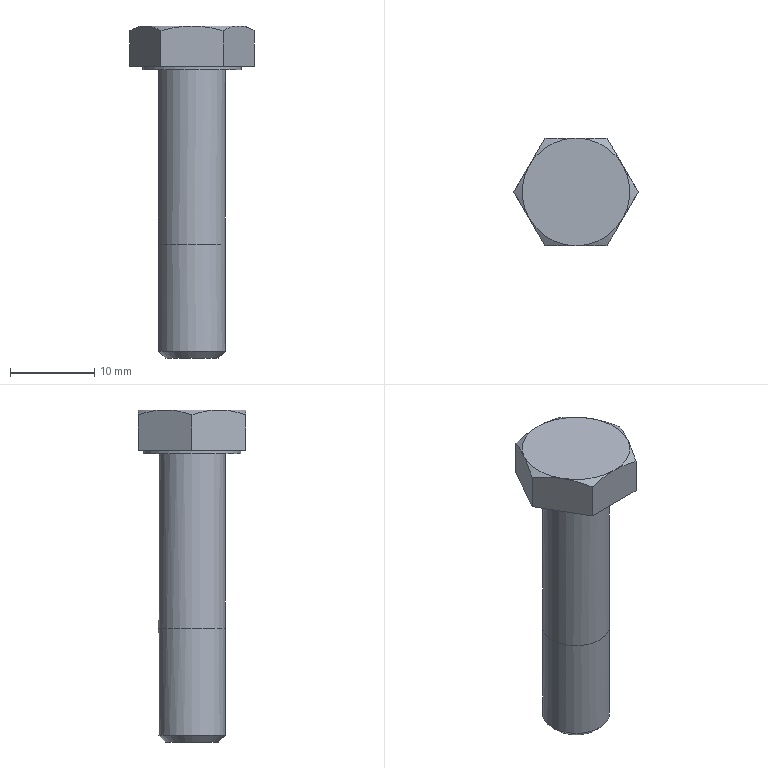Part | NX | features solid 2 | 1 solid | 20 faces | box 14.723 x 12.751 x 39.313 mm | volume 2395 mm3 | plane 10 | cone 7 | cylinder 3 | commonest cylinder face diameters 7.938 x2 11.684 x1
STEP:
#1=CARTESIAN_POINT('',(-3.969,0.,-5.182));
#2=VERTEX_POINT('',#1);
#3=CARTESIAN_POINT('',(0.,0.,-5.182));
#4=DIRECTION('',(0.,0.,-1.));
#5=DIRECTION('',(-1.,0.,0.));
#6=AXIS2_PLACEMENT_3D('',#3,#4,#5);
#7=CIRCLE('',#6,3.969);
#8=EDGE_CURVE('',#2,#2,#7,.T.);
#9=ORIENTED_EDGE('',*,*,#8,.T.);
#10=EDGE_LOOP('',(#9));
#11=FACE_BOUND('',#10,.T.);
#12=CARTESIAN_POINT('',(-3.969,0.,-25.819));
#13=VERTEX_POINT('',#12);
#14=CARTESIAN_POINT('',(-3.11,3.11,-25.819));
#15=CARTESIAN_POINT('',(-4.398,0.,-25.819));
#16=CARTESIAN_POINT('',(-3.11,-3.11,-25.819));
#17=CARTESIAN_POINT('',(0.,-4.398,-25.819));
#18=CARTESIAN_POINT('',(3.11,-3.11,-25.819));
#19=CARTESIAN_POINT('',(4.398,0.,-25.819));
#20=CARTESIAN_POINT('',(3.11,3.11,-25.819));
#21=CARTESIAN_POINT('',(0.,4.398,-25.819));
#22=CARTESIAN_POINT('',(-3.11,3.11,-25.819));
#23=CARTESIAN_POINT('',(-4.398,0.,-25.819));
#24=CARTESIAN_POINT('',(-3.11,-3.11,-25.819));
#25=B_SPLINE_CURVE_WITH_KNOTS('',3,(#14,#15,#16,#17,#18,#19,#20,#21,#22,#23,#24),.UNSPECIFIED.,.T.,.F.,(1,1,1,1,1,1,1,1,1,1,1,1,1,1,1),(-0.375,-0.25,-0.125,0.,0.125,0.25,0.375,0.5,0.625,0.75,0.875,1.,1.125,1.25,1.375),.UNSPECIFIED.);
#26=EDGE_CURVE('',#13,#13,#25,.T.);
#27=ORIENTED_EDGE('',*,*,#26,.T.);
#28=EDGE_LOOP('',(#27));
#29=FACE_BOUND('',#28,.T.);
#30=CARTESIAN_POINT('',(0.,0.,0.));
#31=DIRECTION('',(0.,0.,-1.));
#32=DIRECTION('',(-1.,0.,0.));
#33=AXIS2_PLACEMENT_3D('',#30,#31,#32);
#34=CYLINDRICAL_SURFACE('',#33,3.969);
#35=ADVANCED_FACE('',(#11,#29),#34,.T.);
#36=CARTESIAN_POINT('',(-7.362,0.,-4.775));
#37=VERTEX_POINT('',#36);
#38=CARTESIAN_POINT('',(-3.681,6.375,-4.775));
#39=VERTEX_POINT('',#38);
#40=CARTESIAN_POINT('',(-4.061,5.717,-4.775));
#41=DIRECTION('',(0.5,0.866,0.));
#42=VECTOR('',#41,1000.);
#43=LINE('',#40,#42);
#44=EDGE_CURVE('',#37,#39,#43,.T.);
#45=ORIENTED_EDGE('',*,*,#44,.T.);
#46=CARTESIAN_POINT('',(3.681,6.375,-4.775));
#47=VERTEX_POINT('',#46);
#48=CARTESIAN_POINT('',(5.842,6.375,-4.775));
#49=DIRECTION('',(1.,0.,0.));
#50=VECTOR('',#49,1000.);
#51=LINE('',#48,#50);
#52=EDGE_CURVE('',#39,#47,#51,.T.);
#53=ORIENTED_EDGE('',*,*,#52,.T.);
#54=CARTESIAN_POINT('',(7.362,0.,-4.775));
#55=VERTEX_POINT('',#54);
#56=CARTESIAN_POINT('',(6.982,0.658,-4.775));
#57=DIRECTION('',(0.5,-0.866,0.));
#58=VECTOR('',#57,1000.);
#59=LINE('',#56,#58);
#60=EDGE_CURVE('',#47,#55,#59,.T.);
#61=ORIENTED_EDGE('',*,*,#60,.T.);
#62=CARTESIAN_POINT('',(3.681,-6.375,-4.775));
#63=VERTEX_POINT('',#62);
#64=CARTESIAN_POINT('',(6.982,-0.658,-4.775));
#65=DIRECTION('',(-0.5,-0.866,0.));
#66=VECTOR('',#65,1000.);
#67=LINE('',#64,#66);
#68=EDGE_CURVE('',#55,#63,#67,.T.);
#69=ORIENTED_EDGE('',*,*,#68,.T.);
#70=CARTESIAN_POINT('',(-3.681,-6.375,-4.775));
#71=VERTEX_POINT('',#70);
#72=CARTESIAN_POINT('',(5.842,-6.375,-4.775));
#73=DIRECTION('',(-1.,0.,0.));
#74=VECTOR('',#73,1000.);
#75=LINE('',#72,#74);
#76=EDGE_CURVE('',#63,#71,#75,.T.);
#77=ORIENTED_EDGE('',*,*,#76,.T.);
#78=CARTESIAN_POINT('',(-4.061,-5.717,-4.775));
#79=DIRECTION('',(-0.5,0.866,0.));
#80=VECTOR('',#79,1000.);
#81=LINE('',#78,#80);
#82=EDGE_CURVE('',#71,#37,#81,.T.);
#83=ORIENTED_EDGE('',*,*,#82,.T.);
#84=EDGE_LOOP('',(#45,#53,#61,#69,#77,#83));
#85=FACE_BOUND('',#84,.T.);
#86=CARTESIAN_POINT('',(-5.842,0.,-4.775));
#87=VERTEX_POINT('',#86);
#88=CARTESIAN_POINT('',(0.,0.,-4.775));
#89=DIRECTION('',(0.,0.,-1.));
#90=DIRECTION('',(-1.,0.,0.));
#91=AXIS2_PLACEMENT_3D('',#88,#89,#90);
#92=CIRCLE('',#91,5.842);
#93=EDGE_CURVE('',#87,#87,#92,.T.);
#94=ORIENTED_EDGE('',*,*,#93,.F.);
#95=EDGE_LOOP('',(#94));
#96=FACE_BOUND('',#95,.T.);
#97=CARTESIAN_POINT('',(5.842,0.,-4.775));
#98=DIRECTION('',(0.,0.,-1.));
#99=DIRECTION('',(-1.,0.,0.));
#100=AXIS2_PLACEMENT_3D('',#97,#98,#99);
#101=PLANE('',#100);
#102=ADVANCED_FACE('',(#85,#96),#101,.T.);
#103=CARTESIAN_POINT('',(-3.181,0.,-39.313));
#104=VERTEX_POINT('',#103);
#105=CARTESIAN_POINT('',(0.,0.,-39.313));
#106=DIRECTION('',(0.,0.,-1.));
#107=DIRECTION('',(-1.,0.,0.));
#108=AXIS2_PLACEMENT_3D('',#105,#106,#107);
#109=CIRCLE('',#108,3.181);
#110=EDGE_CURVE('',#104,#104,#109,.T.);
#111=ORIENTED_EDGE('',*,*,#110,.T.);
#112=EDGE_LOOP('',(#111));
#113=FACE_BOUND('',#112,.T.);
#114=CARTESIAN_POINT('',(0.,0.,-39.313));
#115=DIRECTION('',(0.,0.,-1.));
#116=DIRECTION('',(-1.,0.,0.));
#117=AXIS2_PLACEMENT_3D('',#114,#115,#116);
#118=PLANE('',#117);
#119=ADVANCED_FACE('',(#113),#118,.T.);
#120=CARTESIAN_POINT('',(-3.969,0.,-38.525));
#121=VERTEX_POINT('',#120);
#122=CARTESIAN_POINT('',(0.,0.,-38.525));
#123=DIRECTION('',(0.,0.,-1.));
#124=DIRECTION('',(-1.,0.,0.));
#125=AXIS2_PLACEMENT_3D('',#122,#123,#124);
#126=CIRCLE('',#125,3.969);
#127=EDGE_CURVE('',#121,#121,#126,.T.);
#128=ORIENTED_EDGE('',*,*,#127,.T.);
#129=EDGE_LOOP('',(#128));
#130=FACE_BOUND('',#129,.T.);
#131=ORIENTED_EDGE('',*,*,#110,.F.);
#132=EDGE_LOOP('',(#131));
#133=FACE_BOUND('',#132,.T.);
#134=CARTESIAN_POINT('',(0.,0.,-39.313));
#135=DIRECTION('',(0.,0.,1.));
#136=DIRECTION('',(1.,0.,0.));
#137=AXIS2_PLACEMENT_3D('',#134,#135,#136);
#138=CONICAL_SURFACE('',#137,3.181,0.7854);
#139=ADVANCED_FACE('',(#130,#133),#138,.T.);
#140=ORIENTED_EDGE('',*,*,#26,.F.);
#141=EDGE_LOOP('',(#140));
#142=FACE_BOUND('',#141,.T.);
#143=ORIENTED_EDGE('',*,*,#127,.F.);
#144=EDGE_LOOP('',(#143));
#145=FACE_BOUND('',#144,.T.);
#146=CARTESIAN_POINT('',(0.,0.,0.));
#147=DIRECTION('',(0.,0.,-1.));
#148=DIRECTION('',(-1.,0.,0.));
#149=AXIS2_PLACEMENT_3D('',#146,#147,#148);
#150=CYLINDRICAL_SURFACE('',#149,3.969);
#151=ADVANCED_FACE('',(#142,#145),#150,.T.);
#152=CARTESIAN_POINT('',(-5.842,0.,-5.182));
#153=VERTEX_POINT('',#152);
#154=CARTESIAN_POINT('',(0.,0.,-5.182));
#155=DIRECTION('',(0.,0.,-1.));
#156=DIRECTION('',(-1.,0.,0.));
#157=AXIS2_PLACEMENT_3D('',#154,#155,#156);
#158=CIRCLE('',#157,5.842);
#159=EDGE_CURVE('',#153,#153,#158,.T.);
#160=ORIENTED_EDGE('',*,*,#159,.T.);
#161=EDGE_LOOP('',(#160));
#162=FACE_BOUND('',#161,.T.);
#163=ORIENTED_EDGE('',*,*,#8,.F.);
#164=EDGE_LOOP('',(#163));
#165=FACE_BOUND('',#164,.T.);
#166=CARTESIAN_POINT('',(3.969,0.,-5.182));
#167=DIRECTION('',(0.,0.,-1.));
#168=DIRECTION('',(-1.,0.,0.));
#169=AXIS2_PLACEMENT_3D('',#166,#167,#168);
#170=PLANE('',#169);
#171=ADVANCED_FACE('',(#162,#165),#170,.T.);
#172=ORIENTED_EDGE('',*,*,#93,.T.);
#173=EDGE_LOOP('',(#172));
#174=FACE_BOUND('',#173,.T.);
#175=ORIENTED_EDGE('',*,*,#159,.F.);
#176=EDGE_LOOP('',(#175));
#177=FACE_BOUND('',#176,.T.);
#178=CARTESIAN_POINT('',(0.,0.,0.));
#179=DIRECTION('',(0.,0.,-1.));
#180=DIRECTION('',(-1.,0.,0.));
#181=AXIS2_PLACEMENT_3D('',#178,#179,#180);
#182=CYLINDRICAL_SURFACE('',#181,5.842);
#183=ADVANCED_FACE('',(#174,#177),#182,.T.);
#184=ORIENTED_EDGE('',*,*,#52,.F.);
#185=CARTESIAN_POINT('',(-3.681,6.375,-0.5694));
#186=VERTEX_POINT('',#185);
#187=CARTESIAN_POINT('',(-3.681,6.375,-43.244));
#188=DIRECTION('',(0.,0.,1.));
#189=VECTOR('',#188,1000.);
#190=LINE('',#187,#189);
#191=EDGE_CURVE('',#39,#186,#190,.T.);
#192=ORIENTED_EDGE('',*,*,#191,.T.);
#193=CARTESIAN_POINT('',(0.,6.375,0.));
#194=VERTEX_POINT('',#193);
#195=CARTESIAN_POINT('',(-3.681,6.375,-0.5694));
#196=CARTESIAN_POINT('',(-2.484,6.375,-0.2238));
#197=CARTESIAN_POINT('',(-1.244,6.375,0.));
#198=CARTESIAN_POINT('',(0.,6.375,0.));
#199=B_SPLINE_CURVE_WITH_KNOTS('',3,(#195,#196,#197,#198),.UNSPECIFIED.,.F.,.F.,(4,4),(0.006567,0.01029),.UNSPECIFIED.);
#200=EDGE_CURVE('',#194,#186,#199,.F.);
#201=ORIENTED_EDGE('',*,*,#200,.F.);
#202=CARTESIAN_POINT('',(3.681,6.375,-0.5694));
#203=VERTEX_POINT('',#202);
#204=CARTESIAN_POINT('',(0.,6.375,0.));
#205=CARTESIAN_POINT('',(1.245,6.375,0.));
#206=CARTESIAN_POINT('',(2.49,6.375,-0.2258));
#207=CARTESIAN_POINT('',(3.681,6.375,-0.5694));
#208=B_SPLINE_CURVE_WITH_KNOTS('',3,(#204,#205,#206,#207),.UNSPECIFIED.,.F.,.F.,(4,4),(0.01029,0.01402),.UNSPECIFIED.);
#209=EDGE_CURVE('',#203,#194,#208,.F.);
#210=ORIENTED_EDGE('',*,*,#209,.F.);
#211=CARTESIAN_POINT('',(3.681,6.375,-43.244));
#212=DIRECTION('',(0.,0.,1.));
#213=VECTOR('',#212,1000.);
#214=LINE('',#211,#213);
#215=EDGE_CURVE('',#47,#203,#214,.T.);
#216=ORIENTED_EDGE('',*,*,#215,.F.);
#217=EDGE_LOOP('',(#184,#192,#201,#210,#216));
#218=FACE_BOUND('',#217,.T.);
#219=CARTESIAN_POINT('',(3.681,6.375,-43.244));
#220=DIRECTION('',(0.,1.,0.));
#221=DIRECTION('',(0.,0.,1.));
#222=AXIS2_PLACEMENT_3D('',#219,#220,#221);
#223=PLANE('',#222);
#224=ADVANCED_FACE('',(#218),#223,.T.);
#225=ORIENTED_EDGE('',*,*,#44,.F.);
#226=CARTESIAN_POINT('',(-7.362,0.,-0.5694));
#227=VERTEX_POINT('',#226);
#228=CARTESIAN_POINT('',(-7.362,0.,-43.244));
#229=DIRECTION('',(0.,0.,1.));
#230=VECTOR('',#229,1000.);
#231=LINE('',#228,#230);
#232=EDGE_CURVE('',#37,#227,#231,.T.);
#233=ORIENTED_EDGE('',*,*,#232,.T.);
#234=CARTESIAN_POINT('',(-5.521,3.188,0.));
#235=VERTEX_POINT('',#234);
#236=CARTESIAN_POINT('',(-5.521,3.188,0.));
#237=CARTESIAN_POINT('',(-6.146,2.106,0.));
#238=CARTESIAN_POINT('',(-6.761,1.04,-0.2227));
#239=CARTESIAN_POINT('',(-7.362,0.,-0.5694));
#240=B_SPLINE_CURVE_WITH_KNOTS('',3,(#236,#237,#238,#239),.UNSPECIFIED.,.F.,.F.,(4,4),(0.003725,0.007435),.UNSPECIFIED.);
#241=EDGE_CURVE('',#235,#227,#240,.T.);
#242=ORIENTED_EDGE('',*,*,#241,.F.);
#243=CARTESIAN_POINT('',(-3.681,6.375,-0.5694));
#244=CARTESIAN_POINT('',(-4.283,5.332,-0.2218));
#245=CARTESIAN_POINT('',(-4.894,4.274,0.));
#246=CARTESIAN_POINT('',(-5.521,3.188,0.));
#247=B_SPLINE_CURVE_WITH_KNOTS('',3,(#243,#244,#245,#246),.UNSPECIFIED.,.F.,.F.,(4,4),(0.000000238,0.003725),.UNSPECIFIED.);
#248=EDGE_CURVE('',#186,#235,#247,.T.);
#249=ORIENTED_EDGE('',*,*,#248,.F.);
#250=ORIENTED_EDGE('',*,*,#191,.F.);
#251=EDGE_LOOP('',(#225,#233,#242,#249,#250));
#252=FACE_BOUND('',#251,.T.);
#253=CARTESIAN_POINT('',(-3.681,6.375,-43.244));
#254=DIRECTION('',(-0.866,0.5,0.));
#255=DIRECTION('',(-0.5,-0.866,0.));
#256=AXIS2_PLACEMENT_3D('',#253,#254,#255);
#257=PLANE('',#256);
#258=ADVANCED_FACE('',(#252),#257,.T.);
#259=ORIENTED_EDGE('',*,*,#82,.F.);
#260=CARTESIAN_POINT('',(-3.681,-6.375,-0.5694));
#261=VERTEX_POINT('',#260);
#262=CARTESIAN_POINT('',(-3.681,-6.375,-43.244));
#263=DIRECTION('',(0.,0.,1.));
#264=VECTOR('',#263,1000.);
#265=LINE('',#262,#264);
#266=EDGE_CURVE('',#71,#261,#265,.T.);
#267=ORIENTED_EDGE('',*,*,#266,.T.);
#268=CARTESIAN_POINT('',(-5.521,-3.188,0.));
#269=VERTEX_POINT('',#268);
#270=CARTESIAN_POINT('',(-5.521,-3.188,0.));
#271=CARTESIAN_POINT('',(-4.896,-4.27,0.));
#272=CARTESIAN_POINT('',(-4.281,-5.335,-0.2227));
#273=CARTESIAN_POINT('',(-3.681,-6.375,-0.5694));
#274=B_SPLINE_CURVE_WITH_KNOTS('',3,(#270,#271,#272,#273),.UNSPECIFIED.,.F.,.F.,(4,4),(0.003725,0.007435),.UNSPECIFIED.);
#275=EDGE_CURVE('',#269,#261,#274,.T.);
#276=ORIENTED_EDGE('',*,*,#275,.F.);
#277=CARTESIAN_POINT('',(-7.362,0.,-0.5694));
#278=CARTESIAN_POINT('',(-6.76,-1.043,-0.2218));
#279=CARTESIAN_POINT('',(-6.148,-2.102,0.));
#280=CARTESIAN_POINT('',(-5.521,-3.188,0.));
#281=B_SPLINE_CURVE_WITH_KNOTS('',3,(#277,#278,#279,#280),.UNSPECIFIED.,.F.,.F.,(4,4),(0.000000238,0.003725),.UNSPECIFIED.);
#282=EDGE_CURVE('',#227,#269,#281,.T.);
#283=ORIENTED_EDGE('',*,*,#282,.F.);
#284=ORIENTED_EDGE('',*,*,#232,.F.);
#285=EDGE_LOOP('',(#259,#267,#276,#283,#284));
#286=FACE_BOUND('',#285,.T.);
#287=CARTESIAN_POINT('',(-7.362,0.,-43.244));
#288=DIRECTION('',(-0.866,-0.5,0.));
#289=DIRECTION('',(0.5,-0.866,0.));
#290=AXIS2_PLACEMENT_3D('',#287,#288,#289);
#291=PLANE('',#290);
#292=ADVANCED_FACE('',(#286),#291,.T.);
#293=ORIENTED_EDGE('',*,*,#76,.F.);
#294=CARTESIAN_POINT('',(3.681,-6.375,-0.5694));
#295=VERTEX_POINT('',#294);
#296=CARTESIAN_POINT('',(3.681,-6.375,-43.244));
#297=DIRECTION('',(0.,0.,1.));
#298=VECTOR('',#297,1000.);
#299=LINE('',#296,#298);
#300=EDGE_CURVE('',#63,#295,#299,.T.);
#301=ORIENTED_EDGE('',*,*,#300,.T.);
#302=CARTESIAN_POINT('',(0.,-6.375,0.));
#303=VERTEX_POINT('',#302);
#304=CARTESIAN_POINT('',(0.,-6.375,0.));
#305=CARTESIAN_POINT('',(1.245,-6.375,0.));
#306=CARTESIAN_POINT('',(2.49,-6.375,-0.2258));
#307=CARTESIAN_POINT('',(3.681,-6.375,-0.5694));
#308=B_SPLINE_CURVE_WITH_KNOTS('',3,(#304,#305,#306,#307),.UNSPECIFIED.,.F.,.F.,(4,4),(0.01029,0.01402),.UNSPECIFIED.);
#309=EDGE_CURVE('',#303,#295,#308,.T.);
#310=ORIENTED_EDGE('',*,*,#309,.F.);
#311=CARTESIAN_POINT('',(-3.681,-6.375,-0.5694));
#312=CARTESIAN_POINT('',(-2.484,-6.375,-0.2238));
#313=CARTESIAN_POINT('',(-1.244,-6.375,0.));
#314=CARTESIAN_POINT('',(0.,-6.375,0.));
#315=B_SPLINE_CURVE_WITH_KNOTS('',3,(#311,#312,#313,#314),.UNSPECIFIED.,.F.,.F.,(4,4),(0.006567,0.01029),.UNSPECIFIED.);
#316=EDGE_CURVE('',#261,#303,#315,.T.);
#317=ORIENTED_EDGE('',*,*,#316,.F.);
#318=ORIENTED_EDGE('',*,*,#266,.F.);
#319=EDGE_LOOP('',(#293,#301,#310,#317,#318));
#320=FACE_BOUND('',#319,.T.);
#321=CARTESIAN_POINT('',(-3.681,-6.375,-43.244));
#322=DIRECTION('',(0.,-1.,0.));
#323=DIRECTION('',(0.,0.,-1.));
#324=AXIS2_PLACEMENT_3D('',#321,#322,#323);
#325=PLANE('',#324);
#326=ADVANCED_FACE('',(#320),#325,.T.);
#327=ORIENTED_EDGE('',*,*,#68,.F.);
#328=CARTESIAN_POINT('',(7.362,0.,-0.5694));
#329=VERTEX_POINT('',#328);
#330=CARTESIAN_POINT('',(7.362,0.,-43.244));
#331=DIRECTION('',(0.,0.,1.));
#332=VECTOR('',#331,1000.);
#333=LINE('',#330,#332);
#334=EDGE_CURVE('',#55,#329,#333,.T.);
#335=ORIENTED_EDGE('',*,*,#334,.T.);
#336=CARTESIAN_POINT('',(5.521,-3.188,0.));
#337=VERTEX_POINT('',#336);
#338=CARTESIAN_POINT('',(5.521,-3.188,0.));
#339=CARTESIAN_POINT('',(6.146,-2.106,0.));
#340=CARTESIAN_POINT('',(6.761,-1.04,-0.2227));
#341=CARTESIAN_POINT('',(7.362,0.,-0.5694));
#342=B_SPLINE_CURVE_WITH_KNOTS('',3,(#338,#339,#340,#341),.UNSPECIFIED.,.F.,.F.,(4,4),(0.003725,0.007435),.UNSPECIFIED.);
#343=EDGE_CURVE('',#337,#329,#342,.T.);
#344=ORIENTED_EDGE('',*,*,#343,.F.);
#345=CARTESIAN_POINT('',(3.681,-6.375,-0.5694));
#346=CARTESIAN_POINT('',(4.283,-5.332,-0.2218));
#347=CARTESIAN_POINT('',(4.894,-4.274,0.));
#348=CARTESIAN_POINT('',(5.521,-3.188,0.));
#349=B_SPLINE_CURVE_WITH_KNOTS('',3,(#345,#346,#347,#348),.UNSPECIFIED.,.F.,.F.,(4,4),(0.000000238,0.003725),.UNSPECIFIED.);
#350=EDGE_CURVE('',#295,#337,#349,.T.);
#351=ORIENTED_EDGE('',*,*,#350,.F.);
#352=ORIENTED_EDGE('',*,*,#300,.F.);
#353=EDGE_LOOP('',(#327,#335,#344,#351,#352));
#354=FACE_BOUND('',#353,.T.);
#355=CARTESIAN_POINT('',(3.681,-6.375,-43.244));
#356=DIRECTION('',(0.866,-0.5,0.));
#357=DIRECTION('',(0.5,0.866,0.));
#358=AXIS2_PLACEMENT_3D('',#355,#356,#357);
#359=PLANE('',#358);
#360=ADVANCED_FACE('',(#354),#359,.T.);
#361=ORIENTED_EDGE('',*,*,#60,.F.);
#362=ORIENTED_EDGE('',*,*,#215,.T.);
#363=CARTESIAN_POINT('',(5.521,3.188,0.));
#364=VERTEX_POINT('',#363);
#365=CARTESIAN_POINT('',(5.521,3.188,0.));
#366=CARTESIAN_POINT('',(4.896,4.27,0.));
#367=CARTESIAN_POINT('',(4.281,5.335,-0.2227));
#368=CARTESIAN_POINT('',(3.681,6.375,-0.5694));
#369=B_SPLINE_CURVE_WITH_KNOTS('',3,(#365,#366,#367,#368),.UNSPECIFIED.,.F.,.F.,(4,4),(0.003725,0.007435),.UNSPECIFIED.);
#370=EDGE_CURVE('',#364,#203,#369,.T.);
#371=ORIENTED_EDGE('',*,*,#370,.F.);
#372=CARTESIAN_POINT('',(7.362,0.,-0.5694));
#373=CARTESIAN_POINT('',(6.76,1.043,-0.2218));
#374=CARTESIAN_POINT('',(6.148,2.102,0.));
#375=CARTESIAN_POINT('',(5.521,3.188,0.));
#376=B_SPLINE_CURVE_WITH_KNOTS('',3,(#372,#373,#374,#375),.UNSPECIFIED.,.F.,.F.,(4,4),(0.000000238,0.003725),.UNSPECIFIED.);
#377=EDGE_CURVE('',#329,#364,#376,.T.);
#378=ORIENTED_EDGE('',*,*,#377,.F.);
#379=ORIENTED_EDGE('',*,*,#334,.F.);
#380=EDGE_LOOP('',(#361,#362,#371,#378,#379));
#381=FACE_BOUND('',#380,.T.);
#382=CARTESIAN_POINT('',(7.362,0.,-43.244));
#383=DIRECTION('',(0.866,0.5,0.));
#384=DIRECTION('',(-0.5,0.866,0.));
#385=AXIS2_PLACEMENT_3D('',#382,#383,#384);
#386=PLANE('',#385);
#387=ADVANCED_FACE('',(#381),#386,.T.);
#388=CARTESIAN_POINT('',(0.,0.,0.));
#389=DIRECTION('',(0.,0.,-1.));
#390=DIRECTION('',(-1.,0.,0.));
#391=AXIS2_PLACEMENT_3D('',#388,#389,#390);
#392=CIRCLE('',#391,6.375);
#393=EDGE_CURVE('',#364,#337,#392,.T.);
#394=ORIENTED_EDGE('',*,*,#393,.T.);
#395=ORIENTED_EDGE('',*,*,#343,.T.);
#396=ORIENTED_EDGE('',*,*,#377,.T.);
#397=EDGE_LOOP('',(#394,#395,#396));
#398=FACE_BOUND('',#397,.T.);
#399=CARTESIAN_POINT('',(0.,0.,-0.5719));
#400=DIRECTION('',(0.,0.,-1.));
#401=DIRECTION('',(-1.,0.,0.));
#402=AXIS2_PLACEMENT_3D('',#399,#400,#401);
#403=CONICAL_SURFACE('',#402,7.366,1.047);
#404=ADVANCED_FACE('',(#398),#403,.T.);
#405=CARTESIAN_POINT('',(0.,0.,0.));
#406=DIRECTION('',(0.,0.,-1.));
#407=DIRECTION('',(-1.,0.,0.));
#408=AXIS2_PLACEMENT_3D('',#405,#406,#407);
#409=CIRCLE('',#408,6.375);
#410=EDGE_CURVE('',#337,#303,#409,.T.);
#411=ORIENTED_EDGE('',*,*,#410,.T.);
#412=ORIENTED_EDGE('',*,*,#309,.T.);
#413=ORIENTED_EDGE('',*,*,#350,.T.);
#414=EDGE_LOOP('',(#411,#412,#413));
#415=FACE_BOUND('',#414,.T.);
#416=CARTESIAN_POINT('',(0.,0.,-0.5719));
#417=DIRECTION('',(0.,0.,-1.));
#418=DIRECTION('',(-1.,0.,0.));
#419=AXIS2_PLACEMENT_3D('',#416,#417,#418);
#420=CONICAL_SURFACE('',#419,7.366,1.047);
#421=ADVANCED_FACE('',(#415),#420,.T.);
#422=CARTESIAN_POINT('',(0.,0.,0.));
#423=DIRECTION('',(0.,0.,-1.));
#424=DIRECTION('',(-1.,0.,0.));
#425=AXIS2_PLACEMENT_3D('',#422,#423,#424);
#426=CIRCLE('',#425,6.375);
#427=EDGE_CURVE('',#303,#269,#426,.T.);
#428=ORIENTED_EDGE('',*,*,#427,.T.);
#429=ORIENTED_EDGE('',*,*,#275,.T.);
#430=ORIENTED_EDGE('',*,*,#316,.T.);
#431=EDGE_LOOP('',(#428,#429,#430));
#432=FACE_BOUND('',#431,.T.);
#433=CARTESIAN_POINT('',(0.,0.,-0.5719));
#434=DIRECTION('',(0.,0.,-1.));
#435=DIRECTION('',(-1.,0.,0.));
#436=AXIS2_PLACEMENT_3D('',#433,#434,#435);
#437=CONICAL_SURFACE('',#436,7.366,1.047);
#438=ADVANCED_FACE('',(#432),#437,.T.);
#439=CARTESIAN_POINT('',(0.,0.,0.));
#440=DIRECTION('',(0.,0.,-1.));
#441=DIRECTION('',(-1.,0.,0.));
#442=AXIS2_PLACEMENT_3D('',#439,#440,#441);
#443=CIRCLE('',#442,6.375);
#444=EDGE_CURVE('',#269,#235,#443,.T.);
#445=ORIENTED_EDGE('',*,*,#444,.T.);
#446=ORIENTED_EDGE('',*,*,#241,.T.);
#447=ORIENTED_EDGE('',*,*,#282,.T.);
#448=EDGE_LOOP('',(#445,#446,#447));
#449=FACE_BOUND('',#448,.T.);
#450=CARTESIAN_POINT('',(0.,0.,-0.5719));
#451=DIRECTION('',(0.,0.,-1.));
#452=DIRECTION('',(-1.,0.,0.));
#453=AXIS2_PLACEMENT_3D('',#450,#451,#452);
#454=CONICAL_SURFACE('',#453,7.366,1.047);
#455=ADVANCED_FACE('',(#449),#454,.T.);
#456=CARTESIAN_POINT('',(0.,0.,0.));
#457=DIRECTION('',(0.,0.,-1.));
#458=DIRECTION('',(-1.,0.,0.));
#459=AXIS2_PLACEMENT_3D('',#456,#457,#458);
#460=CIRCLE('',#459,6.375);
#461=EDGE_CURVE('',#235,#194,#460,.T.);
#462=ORIENTED_EDGE('',*,*,#461,.T.);
#463=ORIENTED_EDGE('',*,*,#200,.T.);
#464=ORIENTED_EDGE('',*,*,#248,.T.);
#465=EDGE_LOOP('',(#462,#463,#464));
#466=FACE_BOUND('',#465,.T.);
#467=CARTESIAN_POINT('',(0.,0.,-0.5719));
#468=DIRECTION('',(0.,0.,-1.));
#469=DIRECTION('',(-1.,0.,0.));
#470=AXIS2_PLACEMENT_3D('',#467,#468,#469);
#471=CONICAL_SURFACE('',#470,7.366,1.047);
#472=ADVANCED_FACE('',(#466),#471,.T.);
#473=ORIENTED_EDGE('',*,*,#461,.F.);
#474=ORIENTED_EDGE('',*,*,#444,.F.);
#475=ORIENTED_EDGE('',*,*,#427,.F.);
#476=ORIENTED_EDGE('',*,*,#410,.F.);
#477=ORIENTED_EDGE('',*,*,#393,.F.);
#478=CARTESIAN_POINT('',(0.,0.,0.));
#479=DIRECTION('',(0.,0.,-1.));
#480=DIRECTION('',(-1.,0.,0.));
#481=AXIS2_PLACEMENT_3D('',#478,#479,#480);
#482=CIRCLE('',#481,6.375);
#483=EDGE_CURVE('',#194,#364,#482,.T.);
#484=ORIENTED_EDGE('',*,*,#483,.F.);
#485=EDGE_LOOP('',(#473,#474,#475,#476,#477,#484));
#486=FACE_BOUND('',#485,.T.);
#487=CARTESIAN_POINT('',(6.375,0.,0.));
#488=DIRECTION('',(0.,0.,1.));
#489=DIRECTION('',(1.,0.,0.));
#490=AXIS2_PLACEMENT_3D('',#487,#488,#489);
#491=PLANE('',#490);
#492=ADVANCED_FACE('',(#486),#491,.T.);
#493=ORIENTED_EDGE('',*,*,#370,.T.);
#494=ORIENTED_EDGE('',*,*,#209,.T.);
#495=ORIENTED_EDGE('',*,*,#483,.T.);
#496=EDGE_LOOP('',(#493,#494,#495));
#497=FACE_BOUND('',#496,.T.);
#498=CARTESIAN_POINT('',(0.,0.,-0.5719));
#499=DIRECTION('',(0.,0.,-1.));
#500=DIRECTION('',(-1.,0.,0.));
#501=AXIS2_PLACEMENT_3D('',#498,#499,#500);
#502=CONICAL_SURFACE('',#501,7.366,1.047);
#503=ADVANCED_FACE('',(#497),#502,.T.);
#504=CLOSED_SHELL('',(#35,#102,#119,#139,#151,#171,#183,#224,#258,#292,#326,#360,#387,#404,#421,#438,#455,#472,#492,#503));
#505=MANIFOLD_SOLID_BREP('',#504);
#506=(LENGTH_UNIT()NAMED_UNIT(*)SI_UNIT(.MILLI.,.METRE.));
#507=UNCERTAINTY_MEASURE_WITH_UNIT(LENGTH_MEASURE(0.0508),#506,'','');
#508=(NAMED_UNIT(*)PLANE_ANGLE_UNIT()SI_UNIT($,.RADIAN.));
#509=(NAMED_UNIT(*)SI_UNIT($,.STERADIAN.)SOLID_ANGLE_UNIT());
#510=(GEOMETRIC_REPRESENTATION_CONTEXT(3)GLOBAL_UNCERTAINTY_ASSIGNED_CONTEXT((#507))GLOBAL_UNIT_ASSIGNED_CONTEXT((#506,#508,#509))REPRESENTATION_CONTEXT('',''));
#511=ADVANCED_BREP_SHAPE_REPRESENTATION('',(#505),#510);